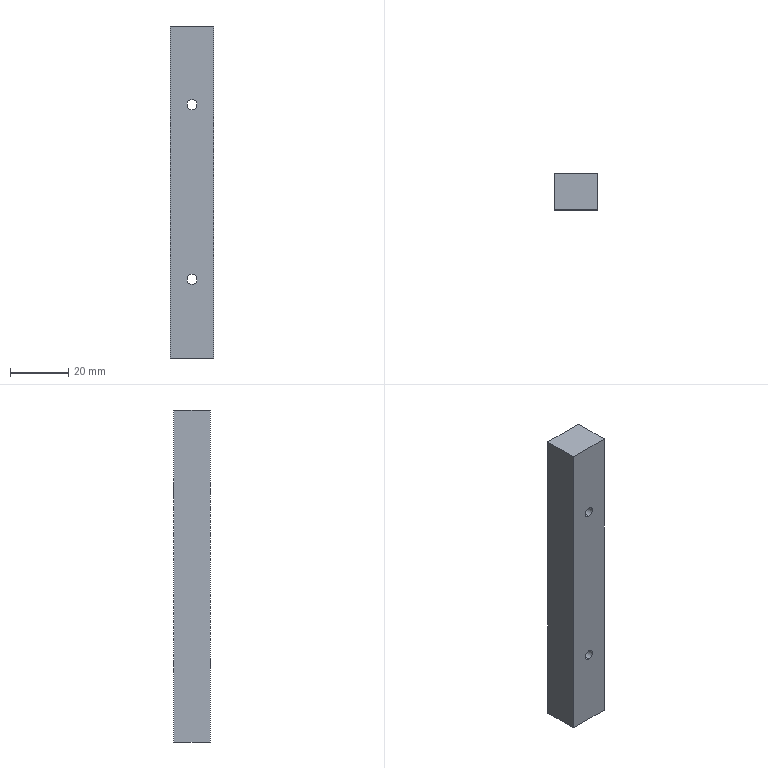Part | STEP file | Bag feed EGH15SA guide rail | 1 solid | 16 faces | box 15 x 12.5 x 114 mm | volume 21017 mm3 | cylinder 8 | plane 8 | commonest cylinder face diameters 3.4 x4 6 x4
STEP:
#1=CARTESIAN_POINT('',(0.,0.,0.));
#2=DIRECTION('',(0.,0.,1.));
#3=DIRECTION('',(1.,0.,0.));
#4=AXIS2_PLACEMENT_3D('',#1,#2,#3);
#5=CARTESIAN_POINT('',(0.,2.85,90.));
#6=VERTEX_POINT('',#5);
#7=CARTESIAN_POINT('',(0.,6.25,90.));
#8=VERTEX_POINT('',#7);
#9=CARTESIAN_POINT('',(0.,6.25,90.));
#10=DIRECTION('',(0.,1.,0.));
#11=VECTOR('',#10,1.);
#12=LINE('',#9,#11);
#13=CARTESIAN_POINT('',(0.,6.25,87.));
#14=DIRECTION('',(0.,1.,0.));
#15=DIRECTION('',(0.,0.,1.));
#16=AXIS2_PLACEMENT_3D('',#13,#14,#15);
#17=CYLINDRICAL_SURFACE('',#16,3.);
#18=CARTESIAN_POINT('',(6.283,0.));
#19=DIRECTION('',(0.,1.));
#20=VECTOR('',#19,1.);
#21=LINE('',#18,#20);
#22=(GEOMETRIC_REPRESENTATION_CONTEXT(2)PARAMETRIC_REPRESENTATION_CONTEXT()REPRESENTATION_CONTEXT('',''));
#23=DEFINITIONAL_REPRESENTATION('',(#21),#22);
#24=PCURVE('',#17,#23);
#25=CARTESIAN_POINT('',(0.,6.25,87.));
#26=DIRECTION('',(0.,1.,0.));
#27=DIRECTION('',(0.,0.,1.));
#28=AXIS2_PLACEMENT_3D('',#25,#26,#27);
#29=CYLINDRICAL_SURFACE('',#28,3.);
#30=CARTESIAN_POINT('',(0.,0.));
#31=DIRECTION('',(0.,1.));
#32=VECTOR('',#31,1.);
#33=LINE('',#30,#32);
#34=(GEOMETRIC_REPRESENTATION_CONTEXT(2)PARAMETRIC_REPRESENTATION_CONTEXT()REPRESENTATION_CONTEXT('',''));
#35=DEFINITIONAL_REPRESENTATION('',(#33),#34);
#36=PCURVE('',#29,#35);
#37=SURFACE_CURVE('',#12,(#24,#36),.PCURVE_S1.);
#38=EDGE_CURVE('',#6,#8,#37,.T.);
#39=ORIENTED_EDGE('',*,*,#38,.T.);
#40=CARTESIAN_POINT('',(0.,6.25,84.));
#41=VERTEX_POINT('',#40);
#42=CARTESIAN_POINT('',(0.,6.25,87.));
#43=DIRECTION('',(0.,1.,0.));
#44=DIRECTION('',(0.,0.,1.));
#45=AXIS2_PLACEMENT_3D('',#42,#43,#44);
#46=CIRCLE('',#45,3.);
#47=CARTESIAN_POINT('',(0.,0.));
#48=DIRECTION('',(1.,0.));
#49=VECTOR('',#48,1.);
#50=LINE('',#47,#49);
#51=(GEOMETRIC_REPRESENTATION_CONTEXT(2)PARAMETRIC_REPRESENTATION_CONTEXT()REPRESENTATION_CONTEXT('',''));
#52=DEFINITIONAL_REPRESENTATION('',(#50),#51);
#53=PCURVE('',#17,#52);
#54=CARTESIAN_POINT('',(-7.5,6.25,114.));
#55=DIRECTION('',(0.,-1.,0.));
#56=DIRECTION('',(0.,0.,-1.));
#57=AXIS2_PLACEMENT_3D('',#54,#55,#56);
#58=PLANE('',#57);
#59=CARTESIAN_POINT('',(24.,7.5));
#60=CARTESIAN_POINT('',(24.,12.696));
#61=CARTESIAN_POINT('',(28.5,10.098));
#62=CARTESIAN_POINT('',(33.,7.5));
#63=CARTESIAN_POINT('',(28.5,4.902));
#64=CARTESIAN_POINT('',(24.,2.304));
#65=CARTESIAN_POINT('',(24.,7.5));
#66=(BOUNDED_CURVE()B_SPLINE_CURVE(2,(#59,#60,#61,#62,#63,#64,#65),.UNSPECIFIED.,.T.,.F.)B_SPLINE_CURVE_WITH_KNOTS((1,2,2,2,2,1),(-2.094,0.,2.094,4.189,6.283,8.378),.UNSPECIFIED.)CURVE()GEOMETRIC_REPRESENTATION_ITEM()RATIONAL_B_SPLINE_CURVE((1.,0.5,1.,0.5,1.,0.5,1.))REPRESENTATION_ITEM(''));
#67=(GEOMETRIC_REPRESENTATION_CONTEXT(2)PARAMETRIC_REPRESENTATION_CONTEXT()REPRESENTATION_CONTEXT('',''));
#68=DEFINITIONAL_REPRESENTATION('',(#66),#67);
#69=PCURVE('',#58,#68);
#70=SURFACE_CURVE('',#46,(#53,#69),.PCURVE_S1.);
#71=EDGE_CURVE('',#41,#8,#70,.T.);
#72=ORIENTED_EDGE('',*,*,#71,.F.);
#73=CARTESIAN_POINT('',(0.,2.85,84.));
#74=VERTEX_POINT('',#73);
#75=CARTESIAN_POINT('',(0.,6.25,84.));
#76=DIRECTION('',(0.,1.,0.));
#77=VECTOR('',#76,1.);
#78=LINE('',#75,#77);
#79=CARTESIAN_POINT('',(3.142,0.));
#80=DIRECTION('',(0.,1.));
#81=VECTOR('',#80,1.);
#82=LINE('',#79,#81);
#83=(GEOMETRIC_REPRESENTATION_CONTEXT(2)PARAMETRIC_REPRESENTATION_CONTEXT()REPRESENTATION_CONTEXT('',''));
#84=DEFINITIONAL_REPRESENTATION('',(#82),#83);
#85=PCURVE('',#17,#84);
#86=CARTESIAN_POINT('',(3.142,0.));
#87=DIRECTION('',(0.,1.));
#88=VECTOR('',#87,1.);
#89=LINE('',#86,#88);
#90=(GEOMETRIC_REPRESENTATION_CONTEXT(2)PARAMETRIC_REPRESENTATION_CONTEXT()REPRESENTATION_CONTEXT('',''));
#91=DEFINITIONAL_REPRESENTATION('',(#89),#90);
#92=PCURVE('',#29,#91);
#93=SURFACE_CURVE('',#78,(#85,#92),.PCURVE_S1.);
#94=EDGE_CURVE('',#74,#41,#93,.T.);
#95=ORIENTED_EDGE('',*,*,#94,.F.);
#96=CARTESIAN_POINT('',(0.,2.85,87.));
#97=DIRECTION('',(0.,1.,0.));
#98=DIRECTION('',(0.,0.,1.));
#99=AXIS2_PLACEMENT_3D('',#96,#97,#98);
#100=CIRCLE('',#99,3.);
#101=CARTESIAN_POINT('',(0.,-3.4));
#102=DIRECTION('',(1.,0.));
#103=VECTOR('',#102,1.);
#104=LINE('',#101,#103);
#105=(GEOMETRIC_REPRESENTATION_CONTEXT(2)PARAMETRIC_REPRESENTATION_CONTEXT()REPRESENTATION_CONTEXT('',''));
#106=DEFINITIONAL_REPRESENTATION('',(#104),#105);
#107=PCURVE('',#17,#106);
#108=CARTESIAN_POINT('',(1.7,2.85,87.));
#109=DIRECTION('',(0.,-1.,0.));
#110=DIRECTION('',(0.,0.,-1.));
#111=AXIS2_PLACEMENT_3D('',#108,#109,#110);
#112=PLANE('',#111);
#113=CARTESIAN_POINT('',(-3.,-1.7));
#114=CARTESIAN_POINT('',(-3.,3.496));
#115=CARTESIAN_POINT('',(1.5,0.8981));
#116=CARTESIAN_POINT('',(6.,-1.7));
#117=CARTESIAN_POINT('',(1.5,-4.298));
#118=CARTESIAN_POINT('',(-3.,-6.896));
#119=CARTESIAN_POINT('',(-3.,-1.7));
#120=(BOUNDED_CURVE()B_SPLINE_CURVE(2,(#113,#114,#115,#116,#117,#118,#119),.UNSPECIFIED.,.T.,.F.)B_SPLINE_CURVE_WITH_KNOTS((1,2,2,2,2,1),(-2.094,0.,2.094,4.189,6.283,8.378),.UNSPECIFIED.)CURVE()GEOMETRIC_REPRESENTATION_ITEM()RATIONAL_B_SPLINE_CURVE((1.,0.5,1.,0.5,1.,0.5,1.))REPRESENTATION_ITEM(''));
#121=(GEOMETRIC_REPRESENTATION_CONTEXT(2)PARAMETRIC_REPRESENTATION_CONTEXT()REPRESENTATION_CONTEXT('',''));
#122=DEFINITIONAL_REPRESENTATION('',(#120),#121);
#123=PCURVE('',#112,#122);
#124=SURFACE_CURVE('',#100,(#107,#123),.PCURVE_S1.);
#125=EDGE_CURVE('',#74,#6,#124,.T.);
#126=ORIENTED_EDGE('',*,*,#125,.T.);
#127=EDGE_LOOP('',(#39,#72,#95,#126));
#128=FACE_BOUND('',#127,.F.);
#129=ADVANCED_FACE('',(#128),#17,.F.);
#130=CARTESIAN_POINT('',(0.,-6.25,88.7));
#131=VERTEX_POINT('',#130);
#132=CARTESIAN_POINT('',(0.,2.85,88.7));
#133=VERTEX_POINT('',#132);
#134=CARTESIAN_POINT('',(0.,6.25,88.7));
#135=DIRECTION('',(0.,1.,0.));
#136=VECTOR('',#135,1.);
#137=LINE('',#134,#136);
#138=CARTESIAN_POINT('',(0.,6.25,87.));
#139=DIRECTION('',(0.,1.,0.));
#140=DIRECTION('',(0.,0.,1.));
#141=AXIS2_PLACEMENT_3D('',#138,#139,#140);
#142=CYLINDRICAL_SURFACE('',#141,1.7);
#143=CARTESIAN_POINT('',(6.283,0.));
#144=DIRECTION('',(0.,1.));
#145=VECTOR('',#144,1.);
#146=LINE('',#143,#145);
#147=(GEOMETRIC_REPRESENTATION_CONTEXT(2)PARAMETRIC_REPRESENTATION_CONTEXT()REPRESENTATION_CONTEXT('',''));
#148=DEFINITIONAL_REPRESENTATION('',(#146),#147);
#149=PCURVE('',#142,#148);
#150=CARTESIAN_POINT('',(0.,6.25,87.));
#151=DIRECTION('',(0.,1.,0.));
#152=DIRECTION('',(0.,0.,1.));
#153=AXIS2_PLACEMENT_3D('',#150,#151,#152);
#154=CYLINDRICAL_SURFACE('',#153,1.7);
#155=CARTESIAN_POINT('',(0.,0.));
#156=DIRECTION('',(0.,1.));
#157=VECTOR('',#156,1.);
#158=LINE('',#155,#157);
#159=(GEOMETRIC_REPRESENTATION_CONTEXT(2)PARAMETRIC_REPRESENTATION_CONTEXT()REPRESENTATION_CONTEXT('',''));
#160=DEFINITIONAL_REPRESENTATION('',(#158),#159);
#161=PCURVE('',#154,#160);
#162=SURFACE_CURVE('',#137,(#149,#161),.PCURVE_S1.);
#163=EDGE_CURVE('',#131,#133,#162,.T.);
#164=ORIENTED_EDGE('',*,*,#163,.T.);
#165=CARTESIAN_POINT('',(0.,2.85,85.3));
#166=VERTEX_POINT('',#165);
#167=CARTESIAN_POINT('',(0.,2.85,87.));
#168=DIRECTION('',(0.,1.,0.));
#169=DIRECTION('',(0.,0.,1.));
#170=AXIS2_PLACEMENT_3D('',#167,#168,#169);
#171=CIRCLE('',#170,1.7);
#172=CARTESIAN_POINT('',(0.,-3.4));
#173=DIRECTION('',(1.,0.));
#174=VECTOR('',#173,1.);
#175=LINE('',#172,#174);
#176=(GEOMETRIC_REPRESENTATION_CONTEXT(2)PARAMETRIC_REPRESENTATION_CONTEXT()REPRESENTATION_CONTEXT('',''));
#177=DEFINITIONAL_REPRESENTATION('',(#175),#176);
#178=PCURVE('',#142,#177);
#179=CARTESIAN_POINT('',(-1.7,-1.7));
#180=CARTESIAN_POINT('',(-1.7,1.244));
#181=CARTESIAN_POINT('',(0.85,-0.2278));
#182=CARTESIAN_POINT('',(3.4,-1.7));
#183=CARTESIAN_POINT('',(0.85,-3.172));
#184=CARTESIAN_POINT('',(-1.7,-4.644));
#185=CARTESIAN_POINT('',(-1.7,-1.7));
#186=(BOUNDED_CURVE()B_SPLINE_CURVE(2,(#179,#180,#181,#182,#183,#184,#185),.UNSPECIFIED.,.T.,.F.)B_SPLINE_CURVE_WITH_KNOTS((1,2,2,2,2,1),(-2.094,0.,2.094,4.189,6.283,8.378),.UNSPECIFIED.)CURVE()GEOMETRIC_REPRESENTATION_ITEM()RATIONAL_B_SPLINE_CURVE((1.,0.5,1.,0.5,1.,0.5,1.))REPRESENTATION_ITEM(''));
#187=(GEOMETRIC_REPRESENTATION_CONTEXT(2)PARAMETRIC_REPRESENTATION_CONTEXT()REPRESENTATION_CONTEXT('',''));
#188=DEFINITIONAL_REPRESENTATION('',(#186),#187);
#189=PCURVE('',#112,#188);
#190=SURFACE_CURVE('',#171,(#178,#189),.PCURVE_S1.);
#191=EDGE_CURVE('',#166,#133,#190,.T.);
#192=ORIENTED_EDGE('',*,*,#191,.F.);
#193=CARTESIAN_POINT('',(0.,-6.25,85.3));
#194=VERTEX_POINT('',#193);
#195=CARTESIAN_POINT('',(0.,6.25,85.3));
#196=DIRECTION('',(0.,1.,0.));
#197=VECTOR('',#196,1.);
#198=LINE('',#195,#197);
#199=CARTESIAN_POINT('',(3.142,0.));
#200=DIRECTION('',(0.,1.));
#201=VECTOR('',#200,1.);
#202=LINE('',#199,#201);
#203=(GEOMETRIC_REPRESENTATION_CONTEXT(2)PARAMETRIC_REPRESENTATION_CONTEXT()REPRESENTATION_CONTEXT('',''));
#204=DEFINITIONAL_REPRESENTATION('',(#202),#203);
#205=PCURVE('',#142,#204);
#206=CARTESIAN_POINT('',(3.142,0.));
#207=DIRECTION('',(0.,1.));
#208=VECTOR('',#207,1.);
#209=LINE('',#206,#208);
#210=(GEOMETRIC_REPRESENTATION_CONTEXT(2)PARAMETRIC_REPRESENTATION_CONTEXT()REPRESENTATION_CONTEXT('',''));
#211=DEFINITIONAL_REPRESENTATION('',(#209),#210);
#212=PCURVE('',#154,#211);
#213=SURFACE_CURVE('',#198,(#205,#212),.PCURVE_S1.);
#214=EDGE_CURVE('',#194,#166,#213,.T.);
#215=ORIENTED_EDGE('',*,*,#214,.F.);
#216=CARTESIAN_POINT('',(0.,-6.25,87.));
#217=DIRECTION('',(0.,1.,0.));
#218=DIRECTION('',(0.,0.,1.));
#219=AXIS2_PLACEMENT_3D('',#216,#217,#218);
#220=CIRCLE('',#219,1.7);
#221=CARTESIAN_POINT('',(0.,-12.5));
#222=DIRECTION('',(1.,0.));
#223=VECTOR('',#222,1.);
#224=LINE('',#221,#223);
#225=(GEOMETRIC_REPRESENTATION_CONTEXT(2)PARAMETRIC_REPRESENTATION_CONTEXT()REPRESENTATION_CONTEXT('',''));
#226=DEFINITIONAL_REPRESENTATION('',(#224),#225);
#227=PCURVE('',#142,#226);
#228=CARTESIAN_POINT('',(-7.5,-6.25,114.));
#229=DIRECTION('',(0.,1.,0.));
#230=DIRECTION('',(0.,0.,1.));
#231=AXIS2_PLACEMENT_3D('',#228,#229,#230);
#232=PLANE('',#231);
#233=CARTESIAN_POINT('',(-27.,7.5));
#234=DIRECTION('',(1.,0.));
#235=AXIS2_PLACEMENT_2D('',#233,#234);
#236=CIRCLE('',#235,1.7);
#237=(GEOMETRIC_REPRESENTATION_CONTEXT(2)PARAMETRIC_REPRESENTATION_CONTEXT()REPRESENTATION_CONTEXT('',''));
#238=DEFINITIONAL_REPRESENTATION('',(#236),#237);
#239=PCURVE('',#232,#238);
#240=SURFACE_CURVE('',#220,(#227,#239),.PCURVE_S1.);
#241=EDGE_CURVE('',#194,#131,#240,.T.);
#242=ORIENTED_EDGE('',*,*,#241,.T.);
#243=EDGE_LOOP('',(#164,#192,#215,#242));
#244=FACE_BOUND('',#243,.F.);
#245=ADVANCED_FACE('',(#244),#142,.F.);
#246=CARTESIAN_POINT('',(0.,2.85,30.));
#247=VERTEX_POINT('',#246);
#248=CARTESIAN_POINT('',(0.,6.25,30.));
#249=VERTEX_POINT('',#248);
#250=CARTESIAN_POINT('',(0.,6.25,30.));
#251=DIRECTION('',(0.,1.,0.));
#252=VECTOR('',#251,1.);
#253=LINE('',#250,#252);
#254=CARTESIAN_POINT('',(0.,6.25,27.));
#255=DIRECTION('',(0.,1.,0.));
#256=DIRECTION('',(0.,0.,1.));
#257=AXIS2_PLACEMENT_3D('',#254,#255,#256);
#258=CYLINDRICAL_SURFACE('',#257,3.);
#259=CARTESIAN_POINT('',(6.283,0.));
#260=DIRECTION('',(0.,1.));
#261=VECTOR('',#260,1.);
#262=LINE('',#259,#261);
#263=(GEOMETRIC_REPRESENTATION_CONTEXT(2)PARAMETRIC_REPRESENTATION_CONTEXT()REPRESENTATION_CONTEXT('',''));
#264=DEFINITIONAL_REPRESENTATION('',(#262),#263);
#265=PCURVE('',#258,#264);
#266=CARTESIAN_POINT('',(0.,6.25,27.));
#267=DIRECTION('',(0.,1.,0.));
#268=DIRECTION('',(0.,0.,1.));
#269=AXIS2_PLACEMENT_3D('',#266,#267,#268);
#270=CYLINDRICAL_SURFACE('',#269,3.);
#271=CARTESIAN_POINT('',(0.,0.));
#272=DIRECTION('',(0.,1.));
#273=VECTOR('',#272,1.);
#274=LINE('',#271,#273);
#275=(GEOMETRIC_REPRESENTATION_CONTEXT(2)PARAMETRIC_REPRESENTATION_CONTEXT()REPRESENTATION_CONTEXT('',''));
#276=DEFINITIONAL_REPRESENTATION('',(#274),#275);
#277=PCURVE('',#270,#276);
#278=SURFACE_CURVE('',#253,(#265,#277),.PCURVE_S1.);
#279=EDGE_CURVE('',#247,#249,#278,.T.);
#280=ORIENTED_EDGE('',*,*,#279,.T.);
#281=CARTESIAN_POINT('',(0.,6.25,24.));
#282=VERTEX_POINT('',#281);
#283=CARTESIAN_POINT('',(0.,6.25,27.));
#284=DIRECTION('',(0.,1.,0.));
#285=DIRECTION('',(0.,0.,1.));
#286=AXIS2_PLACEMENT_3D('',#283,#284,#285);
#287=CIRCLE('',#286,3.);
#288=CARTESIAN_POINT('',(0.,0.));
#289=DIRECTION('',(1.,0.));
#290=VECTOR('',#289,1.);
#291=LINE('',#288,#290);
#292=(GEOMETRIC_REPRESENTATION_CONTEXT(2)PARAMETRIC_REPRESENTATION_CONTEXT()REPRESENTATION_CONTEXT('',''));
#293=DEFINITIONAL_REPRESENTATION('',(#291),#292);
#294=PCURVE('',#258,#293);
#295=CARTESIAN_POINT('',(84.,7.5));
#296=CARTESIAN_POINT('',(84.,12.696));
#297=CARTESIAN_POINT('',(88.5,10.098));
#298=CARTESIAN_POINT('',(93.,7.5));
#299=CARTESIAN_POINT('',(88.5,4.902));
#300=CARTESIAN_POINT('',(84.,2.304));
#301=CARTESIAN_POINT('',(84.,7.5));
#302=(BOUNDED_CURVE()B_SPLINE_CURVE(2,(#295,#296,#297,#298,#299,#300,#301),.UNSPECIFIED.,.T.,.F.)B_SPLINE_CURVE_WITH_KNOTS((1,2,2,2,2,1),(-2.094,0.,2.094,4.189,6.283,8.378),.UNSPECIFIED.)CURVE()GEOMETRIC_REPRESENTATION_ITEM()RATIONAL_B_SPLINE_CURVE((1.,0.5,1.,0.5,1.,0.5,1.))REPRESENTATION_ITEM(''));
#303=(GEOMETRIC_REPRESENTATION_CONTEXT(2)PARAMETRIC_REPRESENTATION_CONTEXT()REPRESENTATION_CONTEXT('',''));
#304=DEFINITIONAL_REPRESENTATION('',(#302),#303);
#305=PCURVE('',#58,#304);
#306=SURFACE_CURVE('',#287,(#294,#305),.PCURVE_S1.);
#307=EDGE_CURVE('',#282,#249,#306,.T.);
#308=ORIENTED_EDGE('',*,*,#307,.F.);
#309=CARTESIAN_POINT('',(0.,2.85,24.));
#310=VERTEX_POINT('',#309);
#311=CARTESIAN_POINT('',(0.,6.25,24.));
#312=DIRECTION('',(0.,1.,0.));
#313=VECTOR('',#312,1.);
#314=LINE('',#311,#313);
#315=CARTESIAN_POINT('',(3.142,0.));
#316=DIRECTION('',(0.,1.));
#317=VECTOR('',#316,1.);
#318=LINE('',#315,#317);
#319=(GEOMETRIC_REPRESENTATION_CONTEXT(2)PARAMETRIC_REPRESENTATION_CONTEXT()REPRESENTATION_CONTEXT('',''));
#320=DEFINITIONAL_REPRESENTATION('',(#318),#319);
#321=PCURVE('',#258,#320);
#322=CARTESIAN_POINT('',(3.142,0.));
#323=DIRECTION('',(0.,1.));
#324=VECTOR('',#323,1.);
#325=LINE('',#322,#324);
#326=(GEOMETRIC_REPRESENTATION_CONTEXT(2)PARAMETRIC_REPRESENTATION_CONTEXT()REPRESENTATION_CONTEXT('',''));
#327=DEFINITIONAL_REPRESENTATION('',(#325),#326);
#328=PCURVE('',#270,#327);
#329=SURFACE_CURVE('',#314,(#321,#328),.PCURVE_S1.);
#330=EDGE_CURVE('',#310,#282,#329,.T.);
#331=ORIENTED_EDGE('',*,*,#330,.F.);
#332=CARTESIAN_POINT('',(0.,2.85,27.));
#333=DIRECTION('',(0.,1.,0.));
#334=DIRECTION('',(0.,0.,1.));
#335=AXIS2_PLACEMENT_3D('',#332,#333,#334);
#336=CIRCLE('',#335,3.);
#337=CARTESIAN_POINT('',(0.,-3.4));
#338=DIRECTION('',(1.,0.));
#339=VECTOR('',#338,1.);
#340=LINE('',#337,#339);
#341=(GEOMETRIC_REPRESENTATION_CONTEXT(2)PARAMETRIC_REPRESENTATION_CONTEXT()REPRESENTATION_CONTEXT('',''));
#342=DEFINITIONAL_REPRESENTATION('',(#340),#341);
#343=PCURVE('',#258,#342);
#344=CARTESIAN_POINT('',(1.7,2.85,27.));
#345=DIRECTION('',(0.,-1.,0.));
#346=DIRECTION('',(0.,0.,-1.));
#347=AXIS2_PLACEMENT_3D('',#344,#345,#346);
#348=PLANE('',#347);
#349=CARTESIAN_POINT('',(-3.,-1.7));
#350=CARTESIAN_POINT('',(-3.,3.496));
#351=CARTESIAN_POINT('',(1.5,0.8981));
#352=CARTESIAN_POINT('',(6.,-1.7));
#353=CARTESIAN_POINT('',(1.5,-4.298));
#354=CARTESIAN_POINT('',(-3.,-6.896));
#355=CARTESIAN_POINT('',(-3.,-1.7));
#356=(BOUNDED_CURVE()B_SPLINE_CURVE(2,(#349,#350,#351,#352,#353,#354,#355),.UNSPECIFIED.,.T.,.F.)B_SPLINE_CURVE_WITH_KNOTS((1,2,2,2,2,1),(-2.094,0.,2.094,4.189,6.283,8.378),.UNSPECIFIED.)CURVE()GEOMETRIC_REPRESENTATION_ITEM()RATIONAL_B_SPLINE_CURVE((1.,0.5,1.,0.5,1.,0.5,1.))REPRESENTATION_ITEM(''));
#357=(GEOMETRIC_REPRESENTATION_CONTEXT(2)PARAMETRIC_REPRESENTATION_CONTEXT()REPRESENTATION_CONTEXT('',''));
#358=DEFINITIONAL_REPRESENTATION('',(#356),#357);
#359=PCURVE('',#348,#358);
#360=SURFACE_CURVE('',#336,(#343,#359),.PCURVE_S1.);
#361=EDGE_CURVE('',#310,#247,#360,.T.);
#362=ORIENTED_EDGE('',*,*,#361,.T.);
#363=EDGE_LOOP('',(#280,#308,#331,#362));
#364=FACE_BOUND('',#363,.F.);
#365=ADVANCED_FACE('',(#364),#258,.F.);
#366=CARTESIAN_POINT('',(0.,-6.25,28.7));
#367=VERTEX_POINT('',#366);
#368=CARTESIAN_POINT('',(0.,2.85,28.7));
#369=VERTEX_POINT('',#368);
#370=CARTESIAN_POINT('',(0.,6.25,28.7));
#371=DIRECTION('',(0.,1.,0.));
#372=VECTOR('',#371,1.);
#373=LINE('',#370,#372);
#374=CARTESIAN_POINT('',(0.,6.25,27.));
#375=DIRECTION('',(0.,1.,0.));
#376=DIRECTION('',(0.,0.,1.));
#377=AXIS2_PLACEMENT_3D('',#374,#375,#376);
#378=CYLINDRICAL_SURFACE('',#377,1.7);
#379=CARTESIAN_POINT('',(6.283,0.));
#380=DIRECTION('',(0.,1.));
#381=VECTOR('',#380,1.);
#382=LINE('',#379,#381);
#383=(GEOMETRIC_REPRESENTATION_CONTEXT(2)PARAMETRIC_REPRESENTATION_CONTEXT()REPRESENTATION_CONTEXT('',''));
#384=DEFINITIONAL_REPRESENTATION('',(#382),#383);
#385=PCURVE('',#378,#384);
#386=CARTESIAN_POINT('',(0.,6.25,27.));
#387=DIRECTION('',(0.,1.,0.));
#388=DIRECTION('',(0.,0.,1.));
#389=AXIS2_PLACEMENT_3D('',#386,#387,#388);
#390=CYLINDRICAL_SURFACE('',#389,1.7);
#391=CARTESIAN_POINT('',(0.,0.));
#392=DIRECTION('',(0.,1.));
#393=VECTOR('',#392,1.);
#394=LINE('',#391,#393);
#395=(GEOMETRIC_REPRESENTATION_CONTEXT(2)PARAMETRIC_REPRESENTATION_CONTEXT()REPRESENTATION_CONTEXT('',''));
#396=DEFINITIONAL_REPRESENTATION('',(#394),#395);
#397=PCURVE('',#390,#396);
#398=SURFACE_CURVE('',#373,(#385,#397),.PCURVE_S1.);
#399=EDGE_CURVE('',#367,#369,#398,.T.);
#400=ORIENTED_EDGE('',*,*,#399,.T.);
#401=CARTESIAN_POINT('',(0.,2.85,25.3));
#402=VERTEX_POINT('',#401);
#403=CARTESIAN_POINT('',(0.,2.85,27.));
#404=DIRECTION('',(0.,1.,0.));
#405=DIRECTION('',(0.,0.,1.));
#406=AXIS2_PLACEMENT_3D('',#403,#404,#405);
#407=CIRCLE('',#406,1.7);
#408=CARTESIAN_POINT('',(0.,-3.4));
#409=DIRECTION('',(1.,0.));
#410=VECTOR('',#409,1.);
#411=LINE('',#408,#410);
#412=(GEOMETRIC_REPRESENTATION_CONTEXT(2)PARAMETRIC_REPRESENTATION_CONTEXT()REPRESENTATION_CONTEXT('',''));
#413=DEFINITIONAL_REPRESENTATION('',(#411),#412);
#414=PCURVE('',#378,#413);
#415=CARTESIAN_POINT('',(-1.7,-1.7));
#416=CARTESIAN_POINT('',(-1.7,1.244));
#417=CARTESIAN_POINT('',(0.85,-0.2278));
#418=CARTESIAN_POINT('',(3.4,-1.7));
#419=CARTESIAN_POINT('',(0.85,-3.172));
#420=CARTESIAN_POINT('',(-1.7,-4.644));
#421=CARTESIAN_POINT('',(-1.7,-1.7));
#422=(BOUNDED_CURVE()B_SPLINE_CURVE(2,(#415,#416,#417,#418,#419,#420,#421),.UNSPECIFIED.,.T.,.F.)B_SPLINE_CURVE_WITH_KNOTS((1,2,2,2,2,1),(-2.094,0.,2.094,4.189,6.283,8.378),.UNSPECIFIED.)CURVE()GEOMETRIC_REPRESENTATION_ITEM()RATIONAL_B_SPLINE_CURVE((1.,0.5,1.,0.5,1.,0.5,1.))REPRESENTATION_ITEM(''));
#423=(GEOMETRIC_REPRESENTATION_CONTEXT(2)PARAMETRIC_REPRESENTATION_CONTEXT()REPRESENTATION_CONTEXT('',''));
#424=DEFINITIONAL_REPRESENTATION('',(#422),#423);
#425=PCURVE('',#348,#424);
#426=SURFACE_CURVE('',#407,(#414,#425),.PCURVE_S1.);
#427=EDGE_CURVE('',#402,#369,#426,.T.);
#428=ORIENTED_EDGE('',*,*,#427,.F.);
#429=CARTESIAN_POINT('',(0.,-6.25,25.3));
#430=VERTEX_POINT('',#429);
#431=CARTESIAN_POINT('',(0.,6.25,25.3));
#432=DIRECTION('',(0.,1.,0.));
#433=VECTOR('',#432,1.);
#434=LINE('',#431,#433);
#435=CARTESIAN_POINT('',(3.142,0.));
#436=DIRECTION('',(0.,1.));
#437=VECTOR('',#436,1.);
#438=LINE('',#435,#437);
#439=(GEOMETRIC_REPRESENTATION_CONTEXT(2)PARAMETRIC_REPRESENTATION_CONTEXT()REPRESENTATION_CONTEXT('',''));
#440=DEFINITIONAL_REPRESENTATION('',(#438),#439);
#441=PCURVE('',#378,#440);
#442=CARTESIAN_POINT('',(3.142,0.));
#443=DIRECTION('',(0.,1.));
#444=VECTOR('',#443,1.);
#445=LINE('',#442,#444);
#446=(GEOMETRIC_REPRESENTATION_CONTEXT(2)PARAMETRIC_REPRESENTATION_CONTEXT()REPRESENTATION_CONTEXT('',''));
#447=DEFINITIONAL_REPRESENTATION('',(#445),#446);
#448=PCURVE('',#390,#447);
#449=SURFACE_CURVE('',#434,(#441,#448),.PCURVE_S1.);
#450=EDGE_CURVE('',#430,#402,#449,.T.);
#451=ORIENTED_EDGE('',*,*,#450,.F.);
#452=CARTESIAN_POINT('',(0.,-6.25,27.));
#453=DIRECTION('',(0.,1.,0.));
#454=DIRECTION('',(0.,0.,1.));
#455=AXIS2_PLACEMENT_3D('',#452,#453,#454);
#456=CIRCLE('',#455,1.7);
#457=CARTESIAN_POINT('',(0.,-12.5));
#458=DIRECTION('',(1.,0.));
#459=VECTOR('',#458,1.);
#460=LINE('',#457,#459);
#461=(GEOMETRIC_REPRESENTATION_CONTEXT(2)PARAMETRIC_REPRESENTATION_CONTEXT()REPRESENTATION_CONTEXT('',''));
#462=DEFINITIONAL_REPRESENTATION('',(#460),#461);
#463=PCURVE('',#378,#462);
#464=CARTESIAN_POINT('',(-87.,7.5));
#465=DIRECTION('',(1.,0.));
#466=AXIS2_PLACEMENT_2D('',#464,#465);
#467=CIRCLE('',#466,1.7);
#468=(GEOMETRIC_REPRESENTATION_CONTEXT(2)PARAMETRIC_REPRESENTATION_CONTEXT()REPRESENTATION_CONTEXT('',''));
#469=DEFINITIONAL_REPRESENTATION('',(#467),#468);
#470=PCURVE('',#232,#469);
#471=SURFACE_CURVE('',#456,(#463,#470),.PCURVE_S1.);
#472=EDGE_CURVE('',#430,#367,#471,.T.);
#473=ORIENTED_EDGE('',*,*,#472,.T.);
#474=EDGE_LOOP('',(#400,#428,#451,#473));
#475=FACE_BOUND('',#474,.F.);
#476=ADVANCED_FACE('',(#475),#378,.F.);
#477=CARTESIAN_POINT('',(7.5,-6.25,0.));
#478=VERTEX_POINT('',#477);
#479=CARTESIAN_POINT('',(7.5,6.25,0.));
#480=VERTEX_POINT('',#479);
#481=CARTESIAN_POINT('',(7.5,-6.25,0.));
#482=DIRECTION('',(0.,1.,0.));
#483=VECTOR('',#482,1.);
#484=LINE('',#481,#483);
#485=CARTESIAN_POINT('',(7.5,-6.25,114.));
#486=DIRECTION('',(-1.,0.,0.));
#487=DIRECTION('',(0.,0.,1.));
#488=AXIS2_PLACEMENT_3D('',#485,#486,#487);
#489=PLANE('',#488);
#490=CARTESIAN_POINT('',(-114.,0.));
#491=DIRECTION('',(0.,1.));
#492=VECTOR('',#491,1.);
#493=LINE('',#490,#492);
#494=(GEOMETRIC_REPRESENTATION_CONTEXT(2)PARAMETRIC_REPRESENTATION_CONTEXT()REPRESENTATION_CONTEXT('',''));
#495=DEFINITIONAL_REPRESENTATION('',(#493),#494);
#496=PCURVE('',#489,#495);
#497=CARTESIAN_POINT('',(0.,0.,0.));
#498=DIRECTION('',(0.,0.,-1.));
#499=DIRECTION('',(-1.,0.,0.));
#500=AXIS2_PLACEMENT_3D('',#497,#498,#499);
#501=PLANE('',#500);
#502=CARTESIAN_POINT('',(-7.5,-6.25));
#503=DIRECTION('',(0.,1.));
#504=VECTOR('',#503,1.);
#505=LINE('',#502,#504);
#506=(GEOMETRIC_REPRESENTATION_CONTEXT(2)PARAMETRIC_REPRESENTATION_CONTEXT()REPRESENTATION_CONTEXT('',''));
#507=DEFINITIONAL_REPRESENTATION('',(#505),#506);
#508=PCURVE('',#501,#507);
#509=SURFACE_CURVE('',#484,(#496,#508),.PCURVE_S1.);
#510=EDGE_CURVE('',#478,#480,#509,.T.);
#511=ORIENTED_EDGE('',*,*,#510,.T.);
#512=CARTESIAN_POINT('',(7.5,6.25,114.));
#513=VERTEX_POINT('',#512);
#514=CARTESIAN_POINT('',(7.5,6.25,114.));
#515=DIRECTION('',(0.,0.,-1.));
#516=VECTOR('',#515,1.);
#517=LINE('',#514,#516);
#518=CARTESIAN_POINT('',(0.,12.5));
#519=DIRECTION('',(-1.,0.));
#520=VECTOR('',#519,1.);
#521=LINE('',#518,#520);
#522=(GEOMETRIC_REPRESENTATION_CONTEXT(2)PARAMETRIC_REPRESENTATION_CONTEXT()REPRESENTATION_CONTEXT('',''));
#523=DEFINITIONAL_REPRESENTATION('',(#521),#522);
#524=PCURVE('',#489,#523);
#525=CARTESIAN_POINT('',(0.,15.));
#526=DIRECTION('',(1.,0.));
#527=VECTOR('',#526,1.);
#528=LINE('',#525,#527);
#529=(GEOMETRIC_REPRESENTATION_CONTEXT(2)PARAMETRIC_REPRESENTATION_CONTEXT()REPRESENTATION_CONTEXT('',''));
#530=DEFINITIONAL_REPRESENTATION('',(#528),#529);
#531=PCURVE('',#58,#530);
#532=SURFACE_CURVE('',#517,(#524,#531),.PCURVE_S1.);
#533=EDGE_CURVE('',#513,#480,#532,.T.);
#534=ORIENTED_EDGE('',*,*,#533,.F.);
#535=CARTESIAN_POINT('',(7.5,-6.25,114.));
#536=VERTEX_POINT('',#535);
#537=CARTESIAN_POINT('',(7.5,-6.25,114.));
#538=DIRECTION('',(0.,1.,0.));
#539=VECTOR('',#538,1.);
#540=LINE('',#537,#539);
#541=CARTESIAN_POINT('',(0.,0.));
#542=DIRECTION('',(0.,1.));
#543=VECTOR('',#542,1.);
#544=LINE('',#541,#543);
#545=(GEOMETRIC_REPRESENTATION_CONTEXT(2)PARAMETRIC_REPRESENTATION_CONTEXT()REPRESENTATION_CONTEXT('',''));
#546=DEFINITIONAL_REPRESENTATION('',(#544),#545);
#547=PCURVE('',#489,#546);
#548=CARTESIAN_POINT('',(0.,0.,114.));
#549=DIRECTION('',(0.,0.,-1.));
#550=DIRECTION('',(-1.,0.,0.));
#551=AXIS2_PLACEMENT_3D('',#548,#549,#550);
#552=PLANE('',#551);
#553=CARTESIAN_POINT('',(-7.5,-6.25));
#554=DIRECTION('',(0.,1.));
#555=VECTOR('',#554,1.);
#556=LINE('',#553,#555);
#557=(GEOMETRIC_REPRESENTATION_CONTEXT(2)PARAMETRIC_REPRESENTATION_CONTEXT()REPRESENTATION_CONTEXT('',''));
#558=DEFINITIONAL_REPRESENTATION('',(#556),#557);
#559=PCURVE('',#552,#558);
#560=SURFACE_CURVE('',#540,(#547,#559),.PCURVE_S1.);
#561=EDGE_CURVE('',#536,#513,#560,.T.);
#562=ORIENTED_EDGE('',*,*,#561,.F.);
#563=CARTESIAN_POINT('',(7.5,-6.25,114.));
#564=DIRECTION('',(0.,0.,-1.));
#565=VECTOR('',#564,1.);
#566=LINE('',#563,#565);
#567=CARTESIAN_POINT('',(0.,0.));
#568=DIRECTION('',(-1.,0.));
#569=VECTOR('',#568,1.);
#570=LINE('',#567,#569);
#571=(GEOMETRIC_REPRESENTATION_CONTEXT(2)PARAMETRIC_REPRESENTATION_CONTEXT()REPRESENTATION_CONTEXT('',''));
#572=DEFINITIONAL_REPRESENTATION('',(#570),#571);
#573=PCURVE('',#489,#572);
#574=CARTESIAN_POINT('',(0.,15.));
#575=DIRECTION('',(-1.,0.));
#576=VECTOR('',#575,1.);
#577=LINE('',#574,#576);
#578=(GEOMETRIC_REPRESENTATION_CONTEXT(2)PARAMETRIC_REPRESENTATION_CONTEXT()REPRESENTATION_CONTEXT('',''));
#579=DEFINITIONAL_REPRESENTATION('',(#577),#578);
#580=PCURVE('',#232,#579);
#581=SURFACE_CURVE('',#566,(#573,#580),.PCURVE_S1.);
#582=EDGE_CURVE('',#536,#478,#581,.T.);
#583=ORIENTED_EDGE('',*,*,#582,.T.);
#584=EDGE_LOOP('',(#511,#534,#562,#583));
#585=FACE_BOUND('',#584,.T.);
#586=ADVANCED_FACE('',(#585),#489,.F.);
#587=CARTESIAN_POINT('',(0.,6.25,87.));
#588=DIRECTION('',(0.,1.,0.));
#589=DIRECTION('',(0.,0.,1.));
#590=AXIS2_PLACEMENT_3D('',#587,#588,#589);
#591=CIRCLE('',#590,3.);
#592=CARTESIAN_POINT('',(24.,7.5));
#593=CARTESIAN_POINT('',(24.,12.696));
#594=CARTESIAN_POINT('',(28.5,10.098));
#595=CARTESIAN_POINT('',(33.,7.5));
#596=CARTESIAN_POINT('',(28.5,4.902));
#597=CARTESIAN_POINT('',(24.,2.304));
#598=CARTESIAN_POINT('',(24.,7.5));
#599=(BOUNDED_CURVE()B_SPLINE_CURVE(2,(#592,#593,#594,#595,#596,#597,#598),.UNSPECIFIED.,.T.,.F.)B_SPLINE_CURVE_WITH_KNOTS((1,2,2,2,2,1),(-2.094,0.,2.094,4.189,6.283,8.378),.UNSPECIFIED.)CURVE()GEOMETRIC_REPRESENTATION_ITEM()RATIONAL_B_SPLINE_CURVE((1.,0.5,1.,0.5,1.,0.5,1.))REPRESENTATION_ITEM(''));
#600=(GEOMETRIC_REPRESENTATION_CONTEXT(2)PARAMETRIC_REPRESENTATION_CONTEXT()REPRESENTATION_CONTEXT('',''));
#601=DEFINITIONAL_REPRESENTATION('',(#599),#600);
#602=PCURVE('',#58,#601);
#603=CARTESIAN_POINT('',(0.,0.));
#604=DIRECTION('',(1.,0.));
#605=VECTOR('',#604,1.);
#606=LINE('',#603,#605);
#607=(GEOMETRIC_REPRESENTATION_CONTEXT(2)PARAMETRIC_REPRESENTATION_CONTEXT()REPRESENTATION_CONTEXT('',''));
#608=DEFINITIONAL_REPRESENTATION('',(#606),#607);
#609=PCURVE('',#29,#608);
#610=SURFACE_CURVE('',#591,(#602,#609),.PCURVE_S1.);
#611=EDGE_CURVE('',#8,#41,#610,.T.);
#612=ORIENTED_EDGE('',*,*,#611,.F.);
#613=ORIENTED_EDGE('',*,*,#71,.F.);
#614=EDGE_LOOP('',(#612,#613));
#615=FACE_BOUND('',#614,.T.);
#616=CARTESIAN_POINT('',(0.,6.25,27.));
#617=DIRECTION('',(0.,1.,0.));
#618=DIRECTION('',(0.,0.,1.));
#619=AXIS2_PLACEMENT_3D('',#616,#617,#618);
#620=CIRCLE('',#619,3.);
#621=CARTESIAN_POINT('',(84.,7.5));
#622=CARTESIAN_POINT('',(84.,12.696));
#623=CARTESIAN_POINT('',(88.5,10.098));
#624=CARTESIAN_POINT('',(93.,7.5));
#625=CARTESIAN_POINT('',(88.5,4.902));
#626=CARTESIAN_POINT('',(84.,2.304));
#627=CARTESIAN_POINT('',(84.,7.5));
#628=(BOUNDED_CURVE()B_SPLINE_CURVE(2,(#621,#622,#623,#624,#625,#626,#627),.UNSPECIFIED.,.T.,.F.)B_SPLINE_CURVE_WITH_KNOTS((1,2,2,2,2,1),(-2.094,0.,2.094,4.189,6.283,8.378),.UNSPECIFIED.)CURVE()GEOMETRIC_REPRESENTATION_ITEM()RATIONAL_B_SPLINE_CURVE((1.,0.5,1.,0.5,1.,0.5,1.))REPRESENTATION_ITEM(''));
#629=(GEOMETRIC_REPRESENTATION_CONTEXT(2)PARAMETRIC_REPRESENTATION_CONTEXT()REPRESENTATION_CONTEXT('',''));
#630=DEFINITIONAL_REPRESENTATION('',(#628),#629);
#631=PCURVE('',#58,#630);
#632=CARTESIAN_POINT('',(0.,0.));
#633=DIRECTION('',(1.,0.));
#634=VECTOR('',#633,1.);
#635=LINE('',#632,#634);
#636=(GEOMETRIC_REPRESENTATION_CONTEXT(2)PARAMETRIC_REPRESENTATION_CONTEXT()REPRESENTATION_CONTEXT('',''));
#637=DEFINITIONAL_REPRESENTATION('',(#635),#636);
#638=PCURVE('',#270,#637);
#639=SURFACE_CURVE('',#620,(#631,#638),.PCURVE_S1.);
#640=EDGE_CURVE('',#249,#282,#639,.T.);
#641=ORIENTED_EDGE('',*,*,#640,.F.);
#642=ORIENTED_EDGE('',*,*,#307,.F.);
#643=EDGE_LOOP('',(#641,#642));
#644=FACE_BOUND('',#643,.T.);
#645=CARTESIAN_POINT('',(-7.5,6.25,0.));
#646=VERTEX_POINT('',#645);
#647=CARTESIAN_POINT('',(-7.5,6.25,0.));
#648=DIRECTION('',(-1.,0.,0.));
#649=VECTOR('',#648,1.);
#650=LINE('',#647,#649);
#651=CARTESIAN_POINT('',(114.,0.));
#652=DIRECTION('',(0.,-1.));
#653=VECTOR('',#652,1.);
#654=LINE('',#651,#653);
#655=(GEOMETRIC_REPRESENTATION_CONTEXT(2)PARAMETRIC_REPRESENTATION_CONTEXT()REPRESENTATION_CONTEXT('',''));
#656=DEFINITIONAL_REPRESENTATION('',(#654),#655);
#657=PCURVE('',#58,#656);
#658=CARTESIAN_POINT('',(7.5,6.25));
#659=DIRECTION('',(1.,0.));
#660=VECTOR('',#659,1.);
#661=LINE('',#658,#660);
#662=(GEOMETRIC_REPRESENTATION_CONTEXT(2)PARAMETRIC_REPRESENTATION_CONTEXT()REPRESENTATION_CONTEXT('',''));
#663=DEFINITIONAL_REPRESENTATION('',(#661),#662);
#664=PCURVE('',#501,#663);
#665=SURFACE_CURVE('',#650,(#657,#664),.PCURVE_S1.);
#666=EDGE_CURVE('',#480,#646,#665,.T.);
#667=ORIENTED_EDGE('',*,*,#666,.T.);
#668=CARTESIAN_POINT('',(-7.5,6.25,114.));
#669=VERTEX_POINT('',#668);
#670=CARTESIAN_POINT('',(-7.5,6.25,114.));
#671=DIRECTION('',(0.,0.,-1.));
#672=VECTOR('',#671,1.);
#673=LINE('',#670,#672);
#674=CARTESIAN_POINT('',(0.,0.));
#675=DIRECTION('',(1.,0.));
#676=VECTOR('',#675,1.);
#677=LINE('',#674,#676);
#678=(GEOMETRIC_REPRESENTATION_CONTEXT(2)PARAMETRIC_REPRESENTATION_CONTEXT()REPRESENTATION_CONTEXT('',''));
#679=DEFINITIONAL_REPRESENTATION('',(#677),#678);
#680=PCURVE('',#58,#679);
#681=CARTESIAN_POINT('',(-7.5,-6.25,114.));
#682=DIRECTION('',(1.,0.,0.));
#683=DIRECTION('',(0.,0.,-1.));
#684=AXIS2_PLACEMENT_3D('',#681,#682,#683);
#685=PLANE('',#684);
#686=CARTESIAN_POINT('',(0.,12.5));
#687=DIRECTION('',(1.,0.));
#688=VECTOR('',#687,1.);
#689=LINE('',#686,#688);
#690=(GEOMETRIC_REPRESENTATION_CONTEXT(2)PARAMETRIC_REPRESENTATION_CONTEXT()REPRESENTATION_CONTEXT('',''));
#691=DEFINITIONAL_REPRESENTATION('',(#689),#690);
#692=PCURVE('',#685,#691);
#693=SURFACE_CURVE('',#673,(#680,#692),.PCURVE_S1.);
#694=EDGE_CURVE('',#669,#646,#693,.T.);
#695=ORIENTED_EDGE('',*,*,#694,.F.);
#696=CARTESIAN_POINT('',(-7.5,6.25,114.));
#697=DIRECTION('',(-1.,0.,0.));
#698=VECTOR('',#697,1.);
#699=LINE('',#696,#698);
#700=CARTESIAN_POINT('',(0.,0.));
#701=DIRECTION('',(0.,-1.));
#702=VECTOR('',#701,1.);
#703=LINE('',#700,#702);
#704=(GEOMETRIC_REPRESENTATION_CONTEXT(2)PARAMETRIC_REPRESENTATION_CONTEXT()REPRESENTATION_CONTEXT('',''));
#705=DEFINITIONAL_REPRESENTATION('',(#703),#704);
#706=PCURVE('',#58,#705);
#707=CARTESIAN_POINT('',(7.5,6.25));
#708=DIRECTION('',(1.,0.));
#709=VECTOR('',#708,1.);
#710=LINE('',#707,#709);
#711=(GEOMETRIC_REPRESENTATION_CONTEXT(2)PARAMETRIC_REPRESENTATION_CONTEXT()REPRESENTATION_CONTEXT('',''));
#712=DEFINITIONAL_REPRESENTATION('',(#710),#711);
#713=PCURVE('',#552,#712);
#714=SURFACE_CURVE('',#699,(#706,#713),.PCURVE_S1.);
#715=EDGE_CURVE('',#513,#669,#714,.T.);
#716=ORIENTED_EDGE('',*,*,#715,.F.);
#717=ORIENTED_EDGE('',*,*,#533,.T.);
#718=EDGE_LOOP('',(#667,#695,#716,#717));
#719=FACE_BOUND('',#718,.T.);
#720=ADVANCED_FACE('',(#615,#644,#719),#58,.F.);
#721=CARTESIAN_POINT('',(-7.5,-6.25,0.));
#722=VERTEX_POINT('',#721);
#723=CARTESIAN_POINT('',(-7.5,-6.25,0.));
#724=DIRECTION('',(0.,-1.,0.));
#725=VECTOR('',#724,1.);
#726=LINE('',#723,#725);
#727=CARTESIAN_POINT('',(114.,0.));
#728=DIRECTION('',(0.,-1.));
#729=VECTOR('',#728,1.);
#730=LINE('',#727,#729);
#731=(GEOMETRIC_REPRESENTATION_CONTEXT(2)PARAMETRIC_REPRESENTATION_CONTEXT()REPRESENTATION_CONTEXT('',''));
#732=DEFINITIONAL_REPRESENTATION('',(#730),#731);
#733=PCURVE('',#685,#732);
#734=CARTESIAN_POINT('',(7.5,-6.25));
#735=DIRECTION('',(0.,-1.));
#736=VECTOR('',#735,1.);
#737=LINE('',#734,#736);
#738=(GEOMETRIC_REPRESENTATION_CONTEXT(2)PARAMETRIC_REPRESENTATION_CONTEXT()REPRESENTATION_CONTEXT('',''));
#739=DEFINITIONAL_REPRESENTATION('',(#737),#738);
#740=PCURVE('',#501,#739);
#741=SURFACE_CURVE('',#726,(#733,#740),.PCURVE_S1.);
#742=EDGE_CURVE('',#646,#722,#741,.T.);
#743=ORIENTED_EDGE('',*,*,#742,.T.);
#744=CARTESIAN_POINT('',(-7.5,-6.25,114.));
#745=VERTEX_POINT('',#744);
#746=CARTESIAN_POINT('',(-7.5,-6.25,114.));
#747=DIRECTION('',(0.,0.,-1.));
#748=VECTOR('',#747,1.);
#749=LINE('',#746,#748);
#750=CARTESIAN_POINT('',(0.,0.));
#751=DIRECTION('',(1.,0.));
#752=VECTOR('',#751,1.);
#753=LINE('',#750,#752);
#754=(GEOMETRIC_REPRESENTATION_CONTEXT(2)PARAMETRIC_REPRESENTATION_CONTEXT()REPRESENTATION_CONTEXT('',''));
#755=DEFINITIONAL_REPRESENTATION('',(#753),#754);
#756=PCURVE('',#685,#755);
#757=CARTESIAN_POINT('',(0.,0.));
#758=DIRECTION('',(-1.,0.));
#759=VECTOR('',#758,1.);
#760=LINE('',#757,#759);
#761=(GEOMETRIC_REPRESENTATION_CONTEXT(2)PARAMETRIC_REPRESENTATION_CONTEXT()REPRESENTATION_CONTEXT('',''));
#762=DEFINITIONAL_REPRESENTATION('',(#760),#761);
#763=PCURVE('',#232,#762);
#764=SURFACE_CURVE('',#749,(#756,#763),.PCURVE_S1.);
#765=EDGE_CURVE('',#745,#722,#764,.T.);
#766=ORIENTED_EDGE('',*,*,#765,.F.);
#767=CARTESIAN_POINT('',(-7.5,-6.25,114.));
#768=DIRECTION('',(0.,-1.,0.));
#769=VECTOR('',#768,1.);
#770=LINE('',#767,#769);
#771=CARTESIAN_POINT('',(0.,0.));
#772=DIRECTION('',(0.,-1.));
#773=VECTOR('',#772,1.);
#774=LINE('',#771,#773);
#775=(GEOMETRIC_REPRESENTATION_CONTEXT(2)PARAMETRIC_REPRESENTATION_CONTEXT()REPRESENTATION_CONTEXT('',''));
#776=DEFINITIONAL_REPRESENTATION('',(#774),#775);
#777=PCURVE('',#685,#776);
#778=CARTESIAN_POINT('',(7.5,-6.25));
#779=DIRECTION('',(0.,-1.));
#780=VECTOR('',#779,1.);
#781=LINE('',#778,#780);
#782=(GEOMETRIC_REPRESENTATION_CONTEXT(2)PARAMETRIC_REPRESENTATION_CONTEXT()REPRESENTATION_CONTEXT('',''));
#783=DEFINITIONAL_REPRESENTATION('',(#781),#782);
#784=PCURVE('',#552,#783);
#785=SURFACE_CURVE('',#770,(#777,#784),.PCURVE_S1.);
#786=EDGE_CURVE('',#669,#745,#785,.T.);
#787=ORIENTED_EDGE('',*,*,#786,.F.);
#788=ORIENTED_EDGE('',*,*,#694,.T.);
#789=EDGE_LOOP('',(#743,#766,#787,#788));
#790=FACE_BOUND('',#789,.T.);
#791=ADVANCED_FACE('',(#790),#685,.F.);
#792=CARTESIAN_POINT('',(0.,-6.25,87.));
#793=DIRECTION('',(0.,1.,0.));
#794=DIRECTION('',(0.,0.,1.));
#795=AXIS2_PLACEMENT_3D('',#792,#793,#794);
#796=CIRCLE('',#795,1.7);
#797=CARTESIAN_POINT('',(-27.,7.5));
#798=DIRECTION('',(1.,0.));
#799=AXIS2_PLACEMENT_2D('',#797,#798);
#800=CIRCLE('',#799,1.7);
#801=(GEOMETRIC_REPRESENTATION_CONTEXT(2)PARAMETRIC_REPRESENTATION_CONTEXT()REPRESENTATION_CONTEXT('',''));
#802=DEFINITIONAL_REPRESENTATION('',(#800),#801);
#803=PCURVE('',#232,#802);
#804=CARTESIAN_POINT('',(0.,-12.5));
#805=DIRECTION('',(1.,0.));
#806=VECTOR('',#805,1.);
#807=LINE('',#804,#806);
#808=(GEOMETRIC_REPRESENTATION_CONTEXT(2)PARAMETRIC_REPRESENTATION_CONTEXT()REPRESENTATION_CONTEXT('',''));
#809=DEFINITIONAL_REPRESENTATION('',(#807),#808);
#810=PCURVE('',#154,#809);
#811=SURFACE_CURVE('',#796,(#803,#810),.PCURVE_S1.);
#812=EDGE_CURVE('',#131,#194,#811,.T.);
#813=ORIENTED_EDGE('',*,*,#812,.T.);
#814=ORIENTED_EDGE('',*,*,#241,.T.);
#815=EDGE_LOOP('',(#813,#814));
#816=FACE_BOUND('',#815,.T.);
#817=CARTESIAN_POINT('',(0.,-6.25,27.));
#818=DIRECTION('',(0.,1.,0.));
#819=DIRECTION('',(0.,0.,1.));
#820=AXIS2_PLACEMENT_3D('',#817,#818,#819);
#821=CIRCLE('',#820,1.7);
#822=CARTESIAN_POINT('',(-87.,7.5));
#823=DIRECTION('',(1.,0.));
#824=AXIS2_PLACEMENT_2D('',#822,#823);
#825=CIRCLE('',#824,1.7);
#826=(GEOMETRIC_REPRESENTATION_CONTEXT(2)PARAMETRIC_REPRESENTATION_CONTEXT()REPRESENTATION_CONTEXT('',''));
#827=DEFINITIONAL_REPRESENTATION('',(#825),#826);
#828=PCURVE('',#232,#827);
#829=CARTESIAN_POINT('',(0.,-12.5));
#830=DIRECTION('',(1.,0.));
#831=VECTOR('',#830,1.);
#832=LINE('',#829,#831);
#833=(GEOMETRIC_REPRESENTATION_CONTEXT(2)PARAMETRIC_REPRESENTATION_CONTEXT()REPRESENTATION_CONTEXT('',''));
#834=DEFINITIONAL_REPRESENTATION('',(#832),#833);
#835=PCURVE('',#390,#834);
#836=SURFACE_CURVE('',#821,(#828,#835),.PCURVE_S1.);
#837=EDGE_CURVE('',#367,#430,#836,.T.);
#838=ORIENTED_EDGE('',*,*,#837,.T.);
#839=ORIENTED_EDGE('',*,*,#472,.T.);
#840=EDGE_LOOP('',(#838,#839));
#841=FACE_BOUND('',#840,.T.);
#842=CARTESIAN_POINT('',(-7.5,-6.25,0.));
#843=DIRECTION('',(1.,0.,0.));
#844=VECTOR('',#843,1.);
#845=LINE('',#842,#844);
#846=CARTESIAN_POINT('',(-114.,0.));
#847=DIRECTION('',(0.,1.));
#848=VECTOR('',#847,1.);
#849=LINE('',#846,#848);
#850=(GEOMETRIC_REPRESENTATION_CONTEXT(2)PARAMETRIC_REPRESENTATION_CONTEXT()REPRESENTATION_CONTEXT('',''));
#851=DEFINITIONAL_REPRESENTATION('',(#849),#850);
#852=PCURVE('',#232,#851);
#853=CARTESIAN_POINT('',(7.5,-6.25));
#854=DIRECTION('',(-1.,0.));
#855=VECTOR('',#854,1.);
#856=LINE('',#853,#855);
#857=(GEOMETRIC_REPRESENTATION_CONTEXT(2)PARAMETRIC_REPRESENTATION_CONTEXT()REPRESENTATION_CONTEXT('',''));
#858=DEFINITIONAL_REPRESENTATION('',(#856),#857);
#859=PCURVE('',#501,#858);
#860=SURFACE_CURVE('',#845,(#852,#859),.PCURVE_S1.);
#861=EDGE_CURVE('',#722,#478,#860,.T.);
#862=ORIENTED_EDGE('',*,*,#861,.T.);
#863=ORIENTED_EDGE('',*,*,#582,.F.);
#864=CARTESIAN_POINT('',(-7.5,-6.25,114.));
#865=DIRECTION('',(1.,0.,0.));
#866=VECTOR('',#865,1.);
#867=LINE('',#864,#866);
#868=CARTESIAN_POINT('',(0.,0.));
#869=DIRECTION('',(0.,1.));
#870=VECTOR('',#869,1.);
#871=LINE('',#868,#870);
#872=(GEOMETRIC_REPRESENTATION_CONTEXT(2)PARAMETRIC_REPRESENTATION_CONTEXT()REPRESENTATION_CONTEXT('',''));
#873=DEFINITIONAL_REPRESENTATION('',(#871),#872);
#874=PCURVE('',#232,#873);
#875=CARTESIAN_POINT('',(7.5,-6.25));
#876=DIRECTION('',(-1.,0.));
#877=VECTOR('',#876,1.);
#878=LINE('',#875,#877);
#879=(GEOMETRIC_REPRESENTATION_CONTEXT(2)PARAMETRIC_REPRESENTATION_CONTEXT()REPRESENTATION_CONTEXT('',''));
#880=DEFINITIONAL_REPRESENTATION('',(#878),#879);
#881=PCURVE('',#552,#880);
#882=SURFACE_CURVE('',#867,(#874,#881),.PCURVE_S1.);
#883=EDGE_CURVE('',#745,#536,#882,.T.);
#884=ORIENTED_EDGE('',*,*,#883,.F.);
#885=ORIENTED_EDGE('',*,*,#765,.T.);
#886=EDGE_LOOP('',(#862,#863,#884,#885));
#887=FACE_BOUND('',#886,.T.);
#888=ADVANCED_FACE('',(#816,#841,#887),#232,.F.);
#889=ORIENTED_EDGE('',*,*,#561,.T.);
#890=ORIENTED_EDGE('',*,*,#715,.T.);
#891=ORIENTED_EDGE('',*,*,#786,.T.);
#892=ORIENTED_EDGE('',*,*,#883,.T.);
#893=EDGE_LOOP('',(#889,#890,#891,#892));
#894=FACE_BOUND('',#893,.T.);
#895=ADVANCED_FACE('',(#894),#552,.F.);
#896=ORIENTED_EDGE('',*,*,#510,.F.);
#897=ORIENTED_EDGE('',*,*,#861,.F.);
#898=ORIENTED_EDGE('',*,*,#742,.F.);
#899=ORIENTED_EDGE('',*,*,#666,.F.);
#900=EDGE_LOOP('',(#896,#897,#898,#899));
#901=FACE_BOUND('',#900,.T.);
#902=ADVANCED_FACE('',(#901),#501,.T.);
#903=CARTESIAN_POINT('',(0.,2.85,27.));
#904=DIRECTION('',(0.,1.,0.));
#905=DIRECTION('',(0.,0.,1.));
#906=AXIS2_PLACEMENT_3D('',#903,#904,#905);
#907=CIRCLE('',#906,1.7);
#908=CARTESIAN_POINT('',(0.,-3.4));
#909=DIRECTION('',(1.,0.));
#910=VECTOR('',#909,1.);
#911=LINE('',#908,#910);
#912=(GEOMETRIC_REPRESENTATION_CONTEXT(2)PARAMETRIC_REPRESENTATION_CONTEXT()REPRESENTATION_CONTEXT('',''));
#913=DEFINITIONAL_REPRESENTATION('',(#911),#912);
#914=PCURVE('',#390,#913);
#915=CARTESIAN_POINT('',(-1.7,-1.7));
#916=CARTESIAN_POINT('',(-1.7,1.244));
#917=CARTESIAN_POINT('',(0.85,-0.2278));
#918=CARTESIAN_POINT('',(3.4,-1.7));
#919=CARTESIAN_POINT('',(0.85,-3.172));
#920=CARTESIAN_POINT('',(-1.7,-4.644));
#921=CARTESIAN_POINT('',(-1.7,-1.7));
#922=(BOUNDED_CURVE()B_SPLINE_CURVE(2,(#915,#916,#917,#918,#919,#920,#921),.UNSPECIFIED.,.T.,.F.)B_SPLINE_CURVE_WITH_KNOTS((1,2,2,2,2,1),(-2.094,0.,2.094,4.189,6.283,8.378),.UNSPECIFIED.)CURVE()GEOMETRIC_REPRESENTATION_ITEM()RATIONAL_B_SPLINE_CURVE((1.,0.5,1.,0.5,1.,0.5,1.))REPRESENTATION_ITEM(''));
#923=(GEOMETRIC_REPRESENTATION_CONTEXT(2)PARAMETRIC_REPRESENTATION_CONTEXT()REPRESENTATION_CONTEXT('',''));
#924=DEFINITIONAL_REPRESENTATION('',(#922),#923);
#925=PCURVE('',#348,#924);
#926=SURFACE_CURVE('',#907,(#914,#925),.PCURVE_S1.);
#927=EDGE_CURVE('',#369,#402,#926,.T.);
#928=ORIENTED_EDGE('',*,*,#927,.F.);
#929=ORIENTED_EDGE('',*,*,#399,.F.);
#930=ORIENTED_EDGE('',*,*,#837,.T.);
#931=ORIENTED_EDGE('',*,*,#450,.T.);
#932=EDGE_LOOP('',(#928,#929,#930,#931));
#933=FACE_BOUND('',#932,.F.);
#934=ADVANCED_FACE('',(#933),#390,.F.);
#935=ORIENTED_EDGE('',*,*,#927,.F.);
#936=ORIENTED_EDGE('',*,*,#427,.F.);
#937=EDGE_LOOP('',(#935,#936));
#938=FACE_BOUND('',#937,.T.);
#939=CARTESIAN_POINT('',(0.,2.85,27.));
#940=DIRECTION('',(0.,1.,0.));
#941=DIRECTION('',(0.,0.,1.));
#942=AXIS2_PLACEMENT_3D('',#939,#940,#941);
#943=CIRCLE('',#942,3.);
#944=CARTESIAN_POINT('',(-3.,-1.7));
#945=CARTESIAN_POINT('',(-3.,3.496));
#946=CARTESIAN_POINT('',(1.5,0.8981));
#947=CARTESIAN_POINT('',(6.,-1.7));
#948=CARTESIAN_POINT('',(1.5,-4.298));
#949=CARTESIAN_POINT('',(-3.,-6.896));
#950=CARTESIAN_POINT('',(-3.,-1.7));
#951=(BOUNDED_CURVE()B_SPLINE_CURVE(2,(#944,#945,#946,#947,#948,#949,#950),.UNSPECIFIED.,.T.,.F.)B_SPLINE_CURVE_WITH_KNOTS((1,2,2,2,2,1),(-2.094,0.,2.094,4.189,6.283,8.378),.UNSPECIFIED.)CURVE()GEOMETRIC_REPRESENTATION_ITEM()RATIONAL_B_SPLINE_CURVE((1.,0.5,1.,0.5,1.,0.5,1.))REPRESENTATION_ITEM(''));
#952=(GEOMETRIC_REPRESENTATION_CONTEXT(2)PARAMETRIC_REPRESENTATION_CONTEXT()REPRESENTATION_CONTEXT('',''));
#953=DEFINITIONAL_REPRESENTATION('',(#951),#952);
#954=PCURVE('',#348,#953);
#955=CARTESIAN_POINT('',(0.,-3.4));
#956=DIRECTION('',(1.,0.));
#957=VECTOR('',#956,1.);
#958=LINE('',#955,#957);
#959=(GEOMETRIC_REPRESENTATION_CONTEXT(2)PARAMETRIC_REPRESENTATION_CONTEXT()REPRESENTATION_CONTEXT('',''));
#960=DEFINITIONAL_REPRESENTATION('',(#958),#959);
#961=PCURVE('',#270,#960);
#962=SURFACE_CURVE('',#943,(#954,#961),.PCURVE_S1.);
#963=EDGE_CURVE('',#247,#310,#962,.T.);
#964=ORIENTED_EDGE('',*,*,#963,.T.);
#965=ORIENTED_EDGE('',*,*,#361,.T.);
#966=EDGE_LOOP('',(#964,#965));
#967=FACE_BOUND('',#966,.T.);
#968=ADVANCED_FACE('',(#938,#967),#348,.F.);
#969=ORIENTED_EDGE('',*,*,#640,.F.);
#970=ORIENTED_EDGE('',*,*,#279,.F.);
#971=ORIENTED_EDGE('',*,*,#963,.T.);
#972=ORIENTED_EDGE('',*,*,#330,.T.);
#973=EDGE_LOOP('',(#969,#970,#971,#972));
#974=FACE_BOUND('',#973,.F.);
#975=ADVANCED_FACE('',(#974),#270,.F.);
#976=CARTESIAN_POINT('',(0.,2.85,87.));
#977=DIRECTION('',(0.,1.,0.));
#978=DIRECTION('',(0.,0.,1.));
#979=AXIS2_PLACEMENT_3D('',#976,#977,#978);
#980=CIRCLE('',#979,1.7);
#981=CARTESIAN_POINT('',(0.,-3.4));
#982=DIRECTION('',(1.,0.));
#983=VECTOR('',#982,1.);
#984=LINE('',#981,#983);
#985=(GEOMETRIC_REPRESENTATION_CONTEXT(2)PARAMETRIC_REPRESENTATION_CONTEXT()REPRESENTATION_CONTEXT('',''));
#986=DEFINITIONAL_REPRESENTATION('',(#984),#985);
#987=PCURVE('',#154,#986);
#988=CARTESIAN_POINT('',(-1.7,-1.7));
#989=CARTESIAN_POINT('',(-1.7,1.244));
#990=CARTESIAN_POINT('',(0.85,-0.2278));
#991=CARTESIAN_POINT('',(3.4,-1.7));
#992=CARTESIAN_POINT('',(0.85,-3.172));
#993=CARTESIAN_POINT('',(-1.7,-4.644));
#994=CARTESIAN_POINT('',(-1.7,-1.7));
#995=(BOUNDED_CURVE()B_SPLINE_CURVE(2,(#988,#989,#990,#991,#992,#993,#994),.UNSPECIFIED.,.T.,.F.)B_SPLINE_CURVE_WITH_KNOTS((1,2,2,2,2,1),(-2.094,0.,2.094,4.189,6.283,8.378),.UNSPECIFIED.)CURVE()GEOMETRIC_REPRESENTATION_ITEM()RATIONAL_B_SPLINE_CURVE((1.,0.5,1.,0.5,1.,0.5,1.))REPRESENTATION_ITEM(''));
#996=(GEOMETRIC_REPRESENTATION_CONTEXT(2)PARAMETRIC_REPRESENTATION_CONTEXT()REPRESENTATION_CONTEXT('',''));
#997=DEFINITIONAL_REPRESENTATION('',(#995),#996);
#998=PCURVE('',#112,#997);
#999=SURFACE_CURVE('',#980,(#987,#998),.PCURVE_S1.);
#1000=EDGE_CURVE('',#133,#166,#999,.T.);
#1001=ORIENTED_EDGE('',*,*,#1000,.F.);
#1002=ORIENTED_EDGE('',*,*,#163,.F.);
#1003=ORIENTED_EDGE('',*,*,#812,.T.);
#1004=ORIENTED_EDGE('',*,*,#214,.T.);
#1005=EDGE_LOOP('',(#1001,#1002,#1003,#1004));
#1006=FACE_BOUND('',#1005,.F.);
#1007=ADVANCED_FACE('',(#1006),#154,.F.);
#1008=ORIENTED_EDGE('',*,*,#1000,.F.);
#1009=ORIENTED_EDGE('',*,*,#191,.F.);
#1010=EDGE_LOOP('',(#1008,#1009));
#1011=FACE_BOUND('',#1010,.T.);
#1012=CARTESIAN_POINT('',(0.,2.85,87.));
#1013=DIRECTION('',(0.,1.,0.));
#1014=DIRECTION('',(0.,0.,1.));
#1015=AXIS2_PLACEMENT_3D('',#1012,#1013,#1014);
#1016=CIRCLE('',#1015,3.);
#1017=CARTESIAN_POINT('',(-3.,-1.7));
#1018=CARTESIAN_POINT('',(-3.,3.496));
#1019=CARTESIAN_POINT('',(1.5,0.8981));
#1020=CARTESIAN_POINT('',(6.,-1.7));
#1021=CARTESIAN_POINT('',(1.5,-4.298));
#1022=CARTESIAN_POINT('',(-3.,-6.896));
#1023=CARTESIAN_POINT('',(-3.,-1.7));
#1024=(BOUNDED_CURVE()B_SPLINE_CURVE(2,(#1017,#1018,#1019,#1020,#1021,#1022,#1023),.UNSPECIFIED.,.T.,.F.)B_SPLINE_CURVE_WITH_KNOTS((1,2,2,2,2,1),(-2.094,0.,2.094,4.189,6.283,8.378),.UNSPECIFIED.)CURVE()GEOMETRIC_REPRESENTATION_ITEM()RATIONAL_B_SPLINE_CURVE((1.,0.5,1.,0.5,1.,0.5,1.))REPRESENTATION_ITEM(''));
#1025=(GEOMETRIC_REPRESENTATION_CONTEXT(2)PARAMETRIC_REPRESENTATION_CONTEXT()REPRESENTATION_CONTEXT('',''));
#1026=DEFINITIONAL_REPRESENTATION('',(#1024),#1025);
#1027=PCURVE('',#112,#1026);
#1028=CARTESIAN_POINT('',(0.,-3.4));
#1029=DIRECTION('',(1.,0.));
#1030=VECTOR('',#1029,1.);
#1031=LINE('',#1028,#1030);
#1032=(GEOMETRIC_REPRESENTATION_CONTEXT(2)PARAMETRIC_REPRESENTATION_CONTEXT()REPRESENTATION_CONTEXT('',''));
#1033=DEFINITIONAL_REPRESENTATION('',(#1031),#1032);
#1034=PCURVE('',#29,#1033);
#1035=SURFACE_CURVE('',#1016,(#1027,#1034),.PCURVE_S1.);
#1036=EDGE_CURVE('',#6,#74,#1035,.T.);
#1037=ORIENTED_EDGE('',*,*,#1036,.T.);
#1038=ORIENTED_EDGE('',*,*,#125,.T.);
#1039=EDGE_LOOP('',(#1037,#1038));
#1040=FACE_BOUND('',#1039,.T.);
#1041=ADVANCED_FACE('',(#1011,#1040),#112,.F.);
#1042=ORIENTED_EDGE('',*,*,#611,.F.);
#1043=ORIENTED_EDGE('',*,*,#38,.F.);
#1044=ORIENTED_EDGE('',*,*,#1036,.T.);
#1045=ORIENTED_EDGE('',*,*,#94,.T.);
#1046=EDGE_LOOP('',(#1042,#1043,#1044,#1045));
#1047=FACE_BOUND('',#1046,.F.);
#1048=ADVANCED_FACE('',(#1047),#29,.F.);
#1049=CLOSED_SHELL('',(#129,#245,#365,#476,#586,#720,#791,#888,#895,#902,#934,#968,#975,#1007,#1041,#1048));
#1050=MANIFOLD_SOLID_BREP('',#1049);
#1051=(LENGTH_UNIT()NAMED_UNIT(*)SI_UNIT(.MILLI.,.METRE.));
#1052=UNCERTAINTY_MEASURE_WITH_UNIT(LENGTH_MEASURE(0.0000001),#1051,'','');
#1053=(NAMED_UNIT(*)PLANE_ANGLE_UNIT()SI_UNIT($,.RADIAN.));
#1054=(NAMED_UNIT(*)SI_UNIT($,.STERADIAN.)SOLID_ANGLE_UNIT());
#1055=(GEOMETRIC_REPRESENTATION_CONTEXT(3)GLOBAL_UNCERTAINTY_ASSIGNED_CONTEXT((#1052))GLOBAL_UNIT_ASSIGNED_CONTEXT((#1051,#1053,#1054))REPRESENTATION_CONTEXT('',''));
#1056=ADVANCED_BREP_SHAPE_REPRESENTATION('',(#4,#1050),#1055);